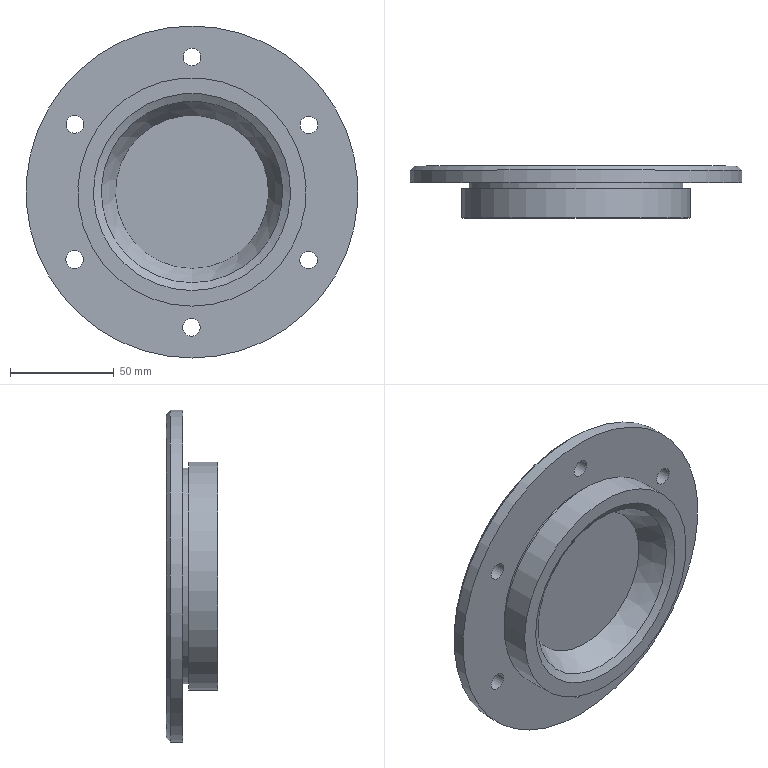Part | NX | features BREP 1, DATUM_CSYS 1 | 1 solid | 19 faces | box 160 x 25 x 160 mm | volume 214879 mm3 | cylinder 9 | plane 6 | cone 4 | commonest cylinder face diameters 8.5 x6 104 x1 110 x1 160 x1
STEP:
#1=CARTESIAN_POINT('',(0.,605.,-36.917));
#2=VERTEX_POINT('',#1);
#3=CARTESIAN_POINT('',(0.,605.,0.));
#4=DIRECTION('',(0.,-1.,0.));
#5=DIRECTION('',(0.,0.,-1.));
#6=AXIS2_PLACEMENT_3D('',#3,#4,#5);
#7=CIRCLE('',#6,36.917);
#8=EDGE_CURVE('',#2,#2,#7,.T.);
#9=ORIENTED_EDGE('',*,*,#8,.F.);
#10=EDGE_LOOP('',(#9));
#11=FACE_BOUND('',#10,.T.);
#12=CARTESIAN_POINT('',(0.,593.165,-43.75));
#13=VERTEX_POINT('',#12);
#14=CARTESIAN_POINT('',(0.,593.165,0.));
#15=DIRECTION('',(0.,-1.,0.));
#16=DIRECTION('',(0.,0.,-1.));
#17=AXIS2_PLACEMENT_3D('',#14,#15,#16);
#18=CIRCLE('',#17,43.75);
#19=EDGE_CURVE('',#13,#13,#18,.T.);
#20=ORIENTED_EDGE('',*,*,#19,.T.);
#21=EDGE_LOOP('',(#20));
#22=FACE_BOUND('',#21,.T.);
#23=CARTESIAN_POINT('',(0.,593.165,0.));
#24=DIRECTION('',(0.,-1.,0.));
#25=DIRECTION('',(0.,0.,-1.));
#26=AXIS2_PLACEMENT_3D('',#23,#24,#25);
#27=CONICAL_SURFACE('',#26,43.75,0.5236);
#28=ADVANCED_FACE('',(#11,#22),#27,.F.);
#29=ORIENTED_EDGE('',*,*,#8,.T.);
#30=EDGE_LOOP('',(#29));
#31=FACE_BOUND('',#30,.T.);
#32=CARTESIAN_POINT('',(36.917,605.,0.));
#33=DIRECTION('',(0.,1.,0.));
#34=DIRECTION('',(0.,0.,1.));
#35=AXIS2_PLACEMENT_3D('',#32,#33,#34);
#36=PLANE('',#35);
#37=ADVANCED_FACE('',(#31),#36,.F.);
#38=CARTESIAN_POINT('',(0.,613.,-51.));
#39=VERTEX_POINT('',#38);
#40=CARTESIAN_POINT('',(0.,613.,0.));
#41=DIRECTION('',(0.,-1.,0.));
#42=DIRECTION('',(0.,0.,-1.));
#43=AXIS2_PLACEMENT_3D('',#40,#41,#42);
#44=CIRCLE('',#43,51.);
#45=EDGE_CURVE('',#39,#39,#44,.T.);
#46=ORIENTED_EDGE('',*,*,#45,.F.);
#47=EDGE_LOOP('',(#46));
#48=FACE_BOUND('',#47,.T.);
#49=CARTESIAN_POINT('',(0.,613.,0.));
#50=DIRECTION('',(0.,-1.,0.));
#51=DIRECTION('',(0.,0.,-1.));
#52=AXIS2_PLACEMENT_3D('',#49,#50,#51);
#53=PLANE('',#52);
#54=ADVANCED_FACE('',(#48),#53,.F.);
#55=CARTESIAN_POINT('',(0.,616.,-54.));
#56=VERTEX_POINT('',#55);
#57=CARTESIAN_POINT('',(0.,616.,0.));
#58=DIRECTION('',(0.,-1.,0.));
#59=DIRECTION('',(0.,0.,-1.));
#60=AXIS2_PLACEMENT_3D('',#57,#58,#59);
#61=CIRCLE('',#60,54.);
#62=EDGE_CURVE('',#56,#56,#61,.T.);
#63=ORIENTED_EDGE('',*,*,#62,.F.);
#64=EDGE_LOOP('',(#63));
#65=FACE_BOUND('',#64,.T.);
#66=ORIENTED_EDGE('',*,*,#45,.T.);
#67=EDGE_LOOP('',(#66));
#68=FACE_BOUND('',#67,.T.);
#69=CARTESIAN_POINT('',(0.,613.,0.));
#70=DIRECTION('',(0.,1.,0.));
#71=DIRECTION('',(0.,0.,1.));
#72=AXIS2_PLACEMENT_3D('',#69,#70,#71);
#73=CONICAL_SURFACE('',#72,51.,0.7854);
#74=ADVANCED_FACE('',(#65,#68),#73,.F.);
#75=CARTESIAN_POINT('',(-56.471,616.,28.317));
#76=VERTEX_POINT('',#75);
#77=CARTESIAN_POINT('',(-56.471,616.,32.567));
#78=DIRECTION('',(0.,-1.,0.));
#79=DIRECTION('',(0.,0.,-1.));
#80=AXIS2_PLACEMENT_3D('',#77,#78,#79);
#81=CIRCLE('',#80,4.25);
#82=EDGE_CURVE('',#76,#76,#81,.F.);
#83=ORIENTED_EDGE('',*,*,#82,.F.);
#84=EDGE_LOOP('',(#83));
#85=FACE_BOUND('',#84,.T.);
#86=CARTESIAN_POINT('',(-0.2963,616.,-69.494));
#87=VERTEX_POINT('',#86);
#88=CARTESIAN_POINT('',(-0.2963,616.,-65.244));
#89=DIRECTION('',(0.,-1.,0.));
#90=DIRECTION('',(0.,0.,-1.));
#91=AXIS2_PLACEMENT_3D('',#88,#89,#90);
#92=CIRCLE('',#91,4.25);
#93=EDGE_CURVE('',#87,#87,#92,.F.);
#94=ORIENTED_EDGE('',*,*,#93,.F.);
#95=EDGE_LOOP('',(#94));
#96=FACE_BOUND('',#95,.T.);
#97=CARTESIAN_POINT('',(0.,616.,60.75));
#98=VERTEX_POINT('',#97);
#99=CARTESIAN_POINT('',(0.,616.,65.));
#100=DIRECTION('',(0.,-1.,0.));
#101=DIRECTION('',(0.,0.,-1.));
#102=AXIS2_PLACEMENT_3D('',#99,#100,#101);
#103=CIRCLE('',#102,4.25);
#104=EDGE_CURVE('',#98,#98,#103,.F.);
#105=ORIENTED_EDGE('',*,*,#104,.F.);
#106=EDGE_LOOP('',(#105));
#107=FACE_BOUND('',#106,.T.);
#108=CARTESIAN_POINT('',(56.175,616.,-37.061));
#109=VERTEX_POINT('',#108);
#110=CARTESIAN_POINT('',(56.175,616.,-32.811));
#111=DIRECTION('',(0.,-1.,0.));
#112=DIRECTION('',(0.,0.,-1.));
#113=AXIS2_PLACEMENT_3D('',#110,#111,#112);
#114=CIRCLE('',#113,4.25);
#115=EDGE_CURVE('',#109,#109,#114,.F.);
#116=ORIENTED_EDGE('',*,*,#115,.F.);
#117=EDGE_LOOP('',(#116));
#118=FACE_BOUND('',#117,.T.);
#119=CARTESIAN_POINT('',(-56.619,616.,-36.805));
#120=VERTEX_POINT('',#119);
#121=CARTESIAN_POINT('',(-56.619,616.,-32.555));
#122=DIRECTION('',(0.,-1.,0.));
#123=DIRECTION('',(0.,0.,-1.));
#124=AXIS2_PLACEMENT_3D('',#121,#122,#123);
#125=CIRCLE('',#124,4.25);
#126=EDGE_CURVE('',#120,#120,#125,.F.);
#127=ORIENTED_EDGE('',*,*,#126,.F.);
#128=EDGE_LOOP('',(#127));
#129=FACE_BOUND('',#128,.T.);
#130=CARTESIAN_POINT('',(56.323,616.,28.061));
#131=VERTEX_POINT('',#130);
#132=CARTESIAN_POINT('',(56.323,616.,32.311));
#133=DIRECTION('',(0.,-1.,0.));
#134=DIRECTION('',(0.,0.,-1.));
#135=AXIS2_PLACEMENT_3D('',#132,#133,#134);
#136=CIRCLE('',#135,4.25);
#137=EDGE_CURVE('',#131,#131,#136,.F.);
#138=ORIENTED_EDGE('',*,*,#137,.F.);
#139=EDGE_LOOP('',(#138));
#140=FACE_BOUND('',#139,.T.);
#141=CARTESIAN_POINT('',(0.,616.,-78.));
#142=VERTEX_POINT('',#141);
#143=CARTESIAN_POINT('',(0.,616.,0.));
#144=DIRECTION('',(0.,-1.,0.));
#145=DIRECTION('',(0.,0.,-1.));
#146=AXIS2_PLACEMENT_3D('',#143,#144,#145);
#147=CIRCLE('',#146,78.);
#148=EDGE_CURVE('',#142,#142,#147,.T.);
#149=ORIENTED_EDGE('',*,*,#148,.F.);
#150=EDGE_LOOP('',(#149));
#151=FACE_BOUND('',#150,.T.);
#152=ORIENTED_EDGE('',*,*,#62,.T.);
#153=EDGE_LOOP('',(#152));
#154=FACE_BOUND('',#153,.T.);
#155=CARTESIAN_POINT('',(54.,616.,0.));
#156=DIRECTION('',(0.,-1.,0.));
#157=DIRECTION('',(0.,0.,-1.));
#158=AXIS2_PLACEMENT_3D('',#155,#156,#157);
#159=PLANE('',#158);
#160=ADVANCED_FACE('',(#85,#96,#107,#118,#129,#140,#151,#154),#159,.F.);
#161=CARTESIAN_POINT('',(0.,614.,-80.));
#162=VERTEX_POINT('',#161);
#163=CARTESIAN_POINT('',(0.,614.,0.));
#164=DIRECTION('',(0.,-1.,0.));
#165=DIRECTION('',(0.,0.,-1.));
#166=AXIS2_PLACEMENT_3D('',#163,#164,#165);
#167=CIRCLE('',#166,80.);
#168=EDGE_CURVE('',#162,#162,#167,.T.);
#169=ORIENTED_EDGE('',*,*,#168,.F.);
#170=EDGE_LOOP('',(#169));
#171=FACE_BOUND('',#170,.T.);
#172=ORIENTED_EDGE('',*,*,#148,.T.);
#173=EDGE_LOOP('',(#172));
#174=FACE_BOUND('',#173,.T.);
#175=CARTESIAN_POINT('',(0.,616.,0.));
#176=DIRECTION('',(0.,-1.,0.));
#177=DIRECTION('',(0.,0.,-1.));
#178=AXIS2_PLACEMENT_3D('',#175,#176,#177);
#179=CONICAL_SURFACE('',#178,78.,0.7854);
#180=ADVANCED_FACE('',(#171,#174),#179,.T.);
#181=CARTESIAN_POINT('',(0.,608.,-80.));
#182=VERTEX_POINT('',#181);
#183=CARTESIAN_POINT('',(0.,608.,0.));
#184=DIRECTION('',(0.,-1.,0.));
#185=DIRECTION('',(0.,0.,-1.));
#186=AXIS2_PLACEMENT_3D('',#183,#184,#185);
#187=CIRCLE('',#186,80.);
#188=EDGE_CURVE('',#182,#182,#187,.T.);
#189=ORIENTED_EDGE('',*,*,#188,.F.);
#190=EDGE_LOOP('',(#189));
#191=FACE_BOUND('',#190,.T.);
#192=ORIENTED_EDGE('',*,*,#168,.T.);
#193=EDGE_LOOP('',(#192));
#194=FACE_BOUND('',#193,.T.);
#195=CARTESIAN_POINT('',(0.,605.,0.));
#196=DIRECTION('',(0.,-1.,0.));
#197=DIRECTION('',(0.,0.,-1.));
#198=AXIS2_PLACEMENT_3D('',#195,#196,#197);
#199=CYLINDRICAL_SURFACE('',#198,80.);
#200=ADVANCED_FACE('',(#191,#194),#199,.T.);
#201=CARTESIAN_POINT('',(-56.471,608.,36.817));
#202=VERTEX_POINT('',#201);
#203=CARTESIAN_POINT('',(-56.471,608.,32.567));
#204=DIRECTION('',(0.,1.,0.));
#205=DIRECTION('',(0.,0.,1.));
#206=AXIS2_PLACEMENT_3D('',#203,#204,#205);
#207=CIRCLE('',#206,4.25);
#208=EDGE_CURVE('',#202,#202,#207,.F.);
#209=ORIENTED_EDGE('',*,*,#208,.F.);
#210=EDGE_LOOP('',(#209));
#211=FACE_BOUND('',#210,.T.);
#212=CARTESIAN_POINT('',(-0.2963,608.,-60.994));
#213=VERTEX_POINT('',#212);
#214=CARTESIAN_POINT('',(-0.2963,608.,-65.244));
#215=DIRECTION('',(0.,1.,0.));
#216=DIRECTION('',(0.,0.,1.));
#217=AXIS2_PLACEMENT_3D('',#214,#215,#216);
#218=CIRCLE('',#217,4.25);
#219=EDGE_CURVE('',#213,#213,#218,.F.);
#220=ORIENTED_EDGE('',*,*,#219,.F.);
#221=EDGE_LOOP('',(#220));
#222=FACE_BOUND('',#221,.T.);
#223=CARTESIAN_POINT('',(0.,608.,69.25));
#224=VERTEX_POINT('',#223);
#225=CARTESIAN_POINT('',(0.,608.,65.));
#226=DIRECTION('',(0.,1.,0.));
#227=DIRECTION('',(0.,0.,1.));
#228=AXIS2_PLACEMENT_3D('',#225,#226,#227);
#229=CIRCLE('',#228,4.25);
#230=EDGE_CURVE('',#224,#224,#229,.F.);
#231=ORIENTED_EDGE('',*,*,#230,.F.);
#232=EDGE_LOOP('',(#231));
#233=FACE_BOUND('',#232,.T.);
#234=CARTESIAN_POINT('',(56.175,608.,-28.561));
#235=VERTEX_POINT('',#234);
#236=CARTESIAN_POINT('',(56.175,608.,-32.811));
#237=DIRECTION('',(0.,1.,0.));
#238=DIRECTION('',(0.,0.,1.));
#239=AXIS2_PLACEMENT_3D('',#236,#237,#238);
#240=CIRCLE('',#239,4.25);
#241=EDGE_CURVE('',#235,#235,#240,.F.);
#242=ORIENTED_EDGE('',*,*,#241,.F.);
#243=EDGE_LOOP('',(#242));
#244=FACE_BOUND('',#243,.T.);
#245=CARTESIAN_POINT('',(-56.619,608.,-28.305));
#246=VERTEX_POINT('',#245);
#247=CARTESIAN_POINT('',(-56.619,608.,-32.555));
#248=DIRECTION('',(0.,1.,0.));
#249=DIRECTION('',(0.,0.,1.));
#250=AXIS2_PLACEMENT_3D('',#247,#248,#249);
#251=CIRCLE('',#250,4.25);
#252=EDGE_CURVE('',#246,#246,#251,.F.);
#253=ORIENTED_EDGE('',*,*,#252,.F.);
#254=EDGE_LOOP('',(#253));
#255=FACE_BOUND('',#254,.T.);
#256=CARTESIAN_POINT('',(56.323,608.,36.561));
#257=VERTEX_POINT('',#256);
#258=CARTESIAN_POINT('',(56.323,608.,32.311));
#259=DIRECTION('',(0.,1.,0.));
#260=DIRECTION('',(0.,0.,1.));
#261=AXIS2_PLACEMENT_3D('',#258,#259,#260);
#262=CIRCLE('',#261,4.25);
#263=EDGE_CURVE('',#257,#257,#262,.F.);
#264=ORIENTED_EDGE('',*,*,#263,.F.);
#265=EDGE_LOOP('',(#264));
#266=FACE_BOUND('',#265,.T.);
#267=CARTESIAN_POINT('',(0.,608.,-52.));
#268=VERTEX_POINT('',#267);
#269=CARTESIAN_POINT('',(0.,608.,0.));
#270=DIRECTION('',(0.,-1.,0.));
#271=DIRECTION('',(0.,0.,-1.));
#272=AXIS2_PLACEMENT_3D('',#269,#270,#271);
#273=CIRCLE('',#272,52.);
#274=EDGE_CURVE('',#268,#268,#273,.T.);
#275=ORIENTED_EDGE('',*,*,#274,.F.);
#276=EDGE_LOOP('',(#275));
#277=FACE_BOUND('',#276,.T.);
#278=ORIENTED_EDGE('',*,*,#188,.T.);
#279=EDGE_LOOP('',(#278));
#280=FACE_BOUND('',#279,.T.);
#281=CARTESIAN_POINT('',(80.,608.,0.));
#282=DIRECTION('',(0.,1.,0.));
#283=DIRECTION('',(0.,0.,1.));
#284=AXIS2_PLACEMENT_3D('',#281,#282,#283);
#285=PLANE('',#284);
#286=ADVANCED_FACE('',(#211,#222,#233,#244,#255,#266,#277,#280),#285,.F.);
#287=CARTESIAN_POINT('',(0.,605.,-52.));
#288=VERTEX_POINT('',#287);
#289=CARTESIAN_POINT('',(0.,605.,0.));
#290=DIRECTION('',(0.,-1.,0.));
#291=DIRECTION('',(0.,0.,-1.));
#292=AXIS2_PLACEMENT_3D('',#289,#290,#291);
#293=CIRCLE('',#292,52.);
#294=EDGE_CURVE('',#288,#288,#293,.T.);
#295=ORIENTED_EDGE('',*,*,#294,.F.);
#296=EDGE_LOOP('',(#295));
#297=FACE_BOUND('',#296,.T.);
#298=ORIENTED_EDGE('',*,*,#274,.T.);
#299=EDGE_LOOP('',(#298));
#300=FACE_BOUND('',#299,.T.);
#301=CARTESIAN_POINT('',(0.,605.,0.));
#302=DIRECTION('',(0.,-1.,0.));
#303=DIRECTION('',(0.,0.,-1.));
#304=AXIS2_PLACEMENT_3D('',#301,#302,#303);
#305=CYLINDRICAL_SURFACE('',#304,52.);
#306=ADVANCED_FACE('',(#297,#300),#305,.T.);
#307=CARTESIAN_POINT('',(0.,605.,-55.));
#308=VERTEX_POINT('',#307);
#309=CARTESIAN_POINT('',(0.,605.,0.));
#310=DIRECTION('',(0.,-1.,0.));
#311=DIRECTION('',(0.,0.,-1.));
#312=AXIS2_PLACEMENT_3D('',#309,#310,#311);
#313=CIRCLE('',#312,55.);
#314=EDGE_CURVE('',#308,#308,#313,.T.);
#315=ORIENTED_EDGE('',*,*,#314,.F.);
#316=EDGE_LOOP('',(#315));
#317=FACE_BOUND('',#316,.T.);
#318=ORIENTED_EDGE('',*,*,#294,.T.);
#319=EDGE_LOOP('',(#318));
#320=FACE_BOUND('',#319,.T.);
#321=CARTESIAN_POINT('',(52.,605.,0.));
#322=DIRECTION('',(0.,-1.,0.));
#323=DIRECTION('',(0.,0.,-1.));
#324=AXIS2_PLACEMENT_3D('',#321,#322,#323);
#325=PLANE('',#324);
#326=ADVANCED_FACE('',(#317,#320),#325,.F.);
#327=CARTESIAN_POINT('',(0.,591.,-55.));
#328=VERTEX_POINT('',#327);
#329=CARTESIAN_POINT('',(0.,591.,0.));
#330=DIRECTION('',(0.,-1.,0.));
#331=DIRECTION('',(0.,0.,-1.));
#332=AXIS2_PLACEMENT_3D('',#329,#330,#331);
#333=CIRCLE('',#332,55.);
#334=EDGE_CURVE('',#328,#328,#333,.T.);
#335=ORIENTED_EDGE('',*,*,#334,.F.);
#336=EDGE_LOOP('',(#335));
#337=FACE_BOUND('',#336,.T.);
#338=ORIENTED_EDGE('',*,*,#314,.T.);
#339=EDGE_LOOP('',(#338));
#340=FACE_BOUND('',#339,.T.);
#341=CARTESIAN_POINT('',(0.,605.,0.));
#342=DIRECTION('',(0.,-1.,0.));
#343=DIRECTION('',(0.,0.,-1.));
#344=AXIS2_PLACEMENT_3D('',#341,#342,#343);
#345=CYLINDRICAL_SURFACE('',#344,55.);
#346=ADVANCED_FACE('',(#337,#340),#345,.T.);
#347=CARTESIAN_POINT('',(0.,591.,-47.5));
#348=VERTEX_POINT('',#347);
#349=CARTESIAN_POINT('',(0.,591.,0.));
#350=DIRECTION('',(0.,-1.,0.));
#351=DIRECTION('',(0.,0.,-1.));
#352=AXIS2_PLACEMENT_3D('',#349,#350,#351);
#353=CIRCLE('',#352,47.5);
#354=EDGE_CURVE('',#348,#348,#353,.T.);
#355=ORIENTED_EDGE('',*,*,#354,.F.);
#356=EDGE_LOOP('',(#355));
#357=FACE_BOUND('',#356,.T.);
#358=ORIENTED_EDGE('',*,*,#334,.T.);
#359=EDGE_LOOP('',(#358));
#360=FACE_BOUND('',#359,.T.);
#361=CARTESIAN_POINT('',(55.,591.,0.));
#362=DIRECTION('',(0.,1.,0.));
#363=DIRECTION('',(0.,0.,1.));
#364=AXIS2_PLACEMENT_3D('',#361,#362,#363);
#365=PLANE('',#364);
#366=ADVANCED_FACE('',(#357,#360),#365,.F.);
#367=ORIENTED_EDGE('',*,*,#19,.F.);
#368=EDGE_LOOP('',(#367));
#369=FACE_BOUND('',#368,.T.);
#370=ORIENTED_EDGE('',*,*,#354,.T.);
#371=EDGE_LOOP('',(#370));
#372=FACE_BOUND('',#371,.T.);
#373=CARTESIAN_POINT('',(0.,591.,0.));
#374=DIRECTION('',(0.,-1.,0.));
#375=DIRECTION('',(0.,0.,-1.));
#376=AXIS2_PLACEMENT_3D('',#373,#374,#375);
#377=CONICAL_SURFACE('',#376,47.5,1.047);
#378=ADVANCED_FACE('',(#369,#372),#377,.F.);
#379=ORIENTED_EDGE('',*,*,#263,.T.);
#380=EDGE_LOOP('',(#379));
#381=FACE_BOUND('',#380,.T.);
#382=ORIENTED_EDGE('',*,*,#137,.T.);
#383=EDGE_LOOP('',(#382));
#384=FACE_BOUND('',#383,.T.);
#385=CARTESIAN_POINT('',(56.323,664.,32.311));
#386=DIRECTION('',(0.,-1.,0.));
#387=DIRECTION('',(0.,0.,-1.));
#388=AXIS2_PLACEMENT_3D('',#385,#386,#387);
#389=CYLINDRICAL_SURFACE('',#388,4.25);
#390=ADVANCED_FACE('',(#381,#384),#389,.F.);
#391=ORIENTED_EDGE('',*,*,#252,.T.);
#392=EDGE_LOOP('',(#391));
#393=FACE_BOUND('',#392,.T.);
#394=ORIENTED_EDGE('',*,*,#126,.T.);
#395=EDGE_LOOP('',(#394));
#396=FACE_BOUND('',#395,.T.);
#397=CARTESIAN_POINT('',(-56.619,664.,-32.555));
#398=DIRECTION('',(0.,-1.,0.));
#399=DIRECTION('',(0.,0.,-1.));
#400=AXIS2_PLACEMENT_3D('',#397,#398,#399);
#401=CYLINDRICAL_SURFACE('',#400,4.25);
#402=ADVANCED_FACE('',(#393,#396),#401,.F.);
#403=ORIENTED_EDGE('',*,*,#241,.T.);
#404=EDGE_LOOP('',(#403));
#405=FACE_BOUND('',#404,.T.);
#406=ORIENTED_EDGE('',*,*,#115,.T.);
#407=EDGE_LOOP('',(#406));
#408=FACE_BOUND('',#407,.T.);
#409=CARTESIAN_POINT('',(56.175,664.,-32.811));
#410=DIRECTION('',(0.,-1.,0.));
#411=DIRECTION('',(0.,0.,-1.));
#412=AXIS2_PLACEMENT_3D('',#409,#410,#411);
#413=CYLINDRICAL_SURFACE('',#412,4.25);
#414=ADVANCED_FACE('',(#405,#408),#413,.F.);
#415=ORIENTED_EDGE('',*,*,#230,.T.);
#416=EDGE_LOOP('',(#415));
#417=FACE_BOUND('',#416,.T.);
#418=ORIENTED_EDGE('',*,*,#104,.T.);
#419=EDGE_LOOP('',(#418));
#420=FACE_BOUND('',#419,.T.);
#421=CARTESIAN_POINT('',(0.,664.,65.));
#422=DIRECTION('',(0.,-1.,0.));
#423=DIRECTION('',(0.,0.,-1.));
#424=AXIS2_PLACEMENT_3D('',#421,#422,#423);
#425=CYLINDRICAL_SURFACE('',#424,4.25);
#426=ADVANCED_FACE('',(#417,#420),#425,.F.);
#427=ORIENTED_EDGE('',*,*,#219,.T.);
#428=EDGE_LOOP('',(#427));
#429=FACE_BOUND('',#428,.T.);
#430=ORIENTED_EDGE('',*,*,#93,.T.);
#431=EDGE_LOOP('',(#430));
#432=FACE_BOUND('',#431,.T.);
#433=CARTESIAN_POINT('',(-0.2963,664.,-65.244));
#434=DIRECTION('',(0.,-1.,0.));
#435=DIRECTION('',(0.,0.,-1.));
#436=AXIS2_PLACEMENT_3D('',#433,#434,#435);
#437=CYLINDRICAL_SURFACE('',#436,4.25);
#438=ADVANCED_FACE('',(#429,#432),#437,.F.);
#439=ORIENTED_EDGE('',*,*,#208,.T.);
#440=EDGE_LOOP('',(#439));
#441=FACE_BOUND('',#440,.T.);
#442=ORIENTED_EDGE('',*,*,#82,.T.);
#443=EDGE_LOOP('',(#442));
#444=FACE_BOUND('',#443,.T.);
#445=CARTESIAN_POINT('',(-56.471,664.,32.567));
#446=DIRECTION('',(0.,-1.,0.));
#447=DIRECTION('',(0.,0.,-1.));
#448=AXIS2_PLACEMENT_3D('',#445,#446,#447);
#449=CYLINDRICAL_SURFACE('',#448,4.25);
#450=ADVANCED_FACE('',(#441,#444),#449,.F.);
#451=CLOSED_SHELL('',(#28,#37,#54,#74,#160,#180,#200,#286,#306,#326,#346,#366,#378,#390,#402,#414,#426,#438,#450));
#452=MANIFOLD_SOLID_BREP('',#451);
#453=(LENGTH_UNIT()NAMED_UNIT(*)SI_UNIT(.MILLI.,.METRE.));
#454=UNCERTAINTY_MEASURE_WITH_UNIT(LENGTH_MEASURE(0.00001),#453,'','');
#455=(NAMED_UNIT(*)PLANE_ANGLE_UNIT()SI_UNIT($,.RADIAN.));
#456=(NAMED_UNIT(*)SI_UNIT($,.STERADIAN.)SOLID_ANGLE_UNIT());
#457=(GEOMETRIC_REPRESENTATION_CONTEXT(3)GLOBAL_UNCERTAINTY_ASSIGNED_CONTEXT((#454))GLOBAL_UNIT_ASSIGNED_CONTEXT((#453,#455,#456))REPRESENTATION_CONTEXT('',''));
#458=ADVANCED_BREP_SHAPE_REPRESENTATION('',(#452),#457);